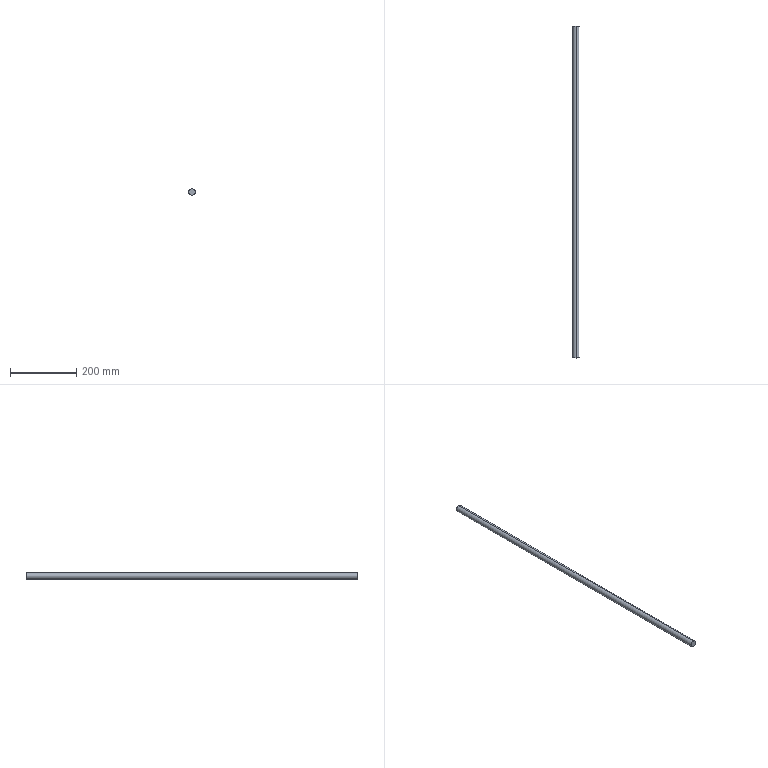Part | SolidWorks | features Extrusion 1 | 1 solid | 4 faces | box 20 x 1000 x 20 mm | volume 314159 mm3 | cylinder 2 | plane 2 | commonest cylinder face diameters 20 x2
STEP:
#1=CARTESIAN_POINT('',(0.,1000.,10.));
#2=VERTEX_POINT('',#1);
#3=CARTESIAN_POINT('',(0.,1000.,-10.));
#4=VERTEX_POINT('',#3);
#5=CARTESIAN_POINT('',(0.,1000.,0.));
#6=DIRECTION('',(0.,1.,0.));
#7=DIRECTION('',(0.,0.,1.));
#8=AXIS2_PLACEMENT_3D('',#5,#6,#7);
#9=CIRCLE('',#8,10.);
#10=EDGE_CURVE('',#2,#4,#9,.T.);
#11=ORIENTED_EDGE('',*,*,#10,.F.);
#12=CARTESIAN_POINT('',(0.,0.,10.));
#13=VERTEX_POINT('',#12);
#14=CARTESIAN_POINT('',(0.,1000.,10.));
#15=DIRECTION('',(0.,-1.,0.));
#16=VECTOR('',#15,1000.);
#17=LINE('',#14,#16);
#18=EDGE_CURVE('',#2,#13,#17,.T.);
#19=ORIENTED_EDGE('',*,*,#18,.T.);
#20=CARTESIAN_POINT('',(0.,0.,-10.));
#21=VERTEX_POINT('',#20);
#22=CARTESIAN_POINT('',(0.,0.,0.));
#23=DIRECTION('',(0.,1.,0.));
#24=DIRECTION('',(0.,0.,1.));
#25=AXIS2_PLACEMENT_3D('',#22,#23,#24);
#26=CIRCLE('',#25,10.);
#27=EDGE_CURVE('',#13,#21,#26,.T.);
#28=ORIENTED_EDGE('',*,*,#27,.T.);
#29=CARTESIAN_POINT('',(0.,1000.,-10.));
#30=DIRECTION('',(0.,-1.,0.));
#31=VECTOR('',#30,1000.);
#32=LINE('',#29,#31);
#33=EDGE_CURVE('',#4,#21,#32,.T.);
#34=ORIENTED_EDGE('',*,*,#33,.F.);
#35=EDGE_LOOP('',(#11,#19,#28,#34));
#36=FACE_OUTER_BOUND('',#35,.T.);
#37=CARTESIAN_POINT('',(0.,1000.,0.));
#38=DIRECTION('',(0.,-1.,0.));
#39=DIRECTION('',(0.,0.,-1.));
#40=AXIS2_PLACEMENT_3D('',#37,#38,#39);
#41=CYLINDRICAL_SURFACE('',#40,10.);
#42=ADVANCED_FACE('',(#36),#41,.T.);
#43=ORIENTED_EDGE('',*,*,#18,.F.);
#44=CARTESIAN_POINT('',(0.,1000.,0.));
#45=DIRECTION('',(0.,1.,0.));
#46=DIRECTION('',(0.,0.,1.));
#47=AXIS2_PLACEMENT_3D('',#44,#45,#46);
#48=CIRCLE('',#47,10.);
#49=EDGE_CURVE('',#4,#2,#48,.T.);
#50=ORIENTED_EDGE('',*,*,#49,.F.);
#51=ORIENTED_EDGE('',*,*,#33,.T.);
#52=CARTESIAN_POINT('',(0.,0.,0.));
#53=DIRECTION('',(0.,1.,0.));
#54=DIRECTION('',(0.,0.,1.));
#55=AXIS2_PLACEMENT_3D('',#52,#53,#54);
#56=CIRCLE('',#55,10.);
#57=EDGE_CURVE('',#21,#13,#56,.T.);
#58=ORIENTED_EDGE('',*,*,#57,.T.);
#59=EDGE_LOOP('',(#43,#50,#51,#58));
#60=FACE_OUTER_BOUND('',#59,.T.);
#61=CARTESIAN_POINT('',(0.,1000.,0.));
#62=DIRECTION('',(0.,-1.,0.));
#63=DIRECTION('',(0.,0.,-1.));
#64=AXIS2_PLACEMENT_3D('',#61,#62,#63);
#65=CYLINDRICAL_SURFACE('',#64,10.);
#66=ADVANCED_FACE('',(#60),#65,.T.);
#67=ORIENTED_EDGE('',*,*,#49,.T.);
#68=ORIENTED_EDGE('',*,*,#10,.T.);
#69=EDGE_LOOP('',(#67,#68));
#70=FACE_OUTER_BOUND('',#69,.T.);
#71=CARTESIAN_POINT('',(0.,1000.,0.));
#72=DIRECTION('',(0.,1.,0.));
#73=DIRECTION('',(0.,0.,1.));
#74=AXIS2_PLACEMENT_3D('',#71,#72,#73);
#75=PLANE('',#74);
#76=ADVANCED_FACE('',(#70),#75,.T.);
#77=ORIENTED_EDGE('',*,*,#57,.F.);
#78=ORIENTED_EDGE('',*,*,#27,.F.);
#79=EDGE_LOOP('',(#77,#78));
#80=FACE_OUTER_BOUND('',#79,.T.);
#81=CARTESIAN_POINT('',(0.,0.,0.));
#82=DIRECTION('',(0.,1.,0.));
#83=DIRECTION('',(0.,0.,1.));
#84=AXIS2_PLACEMENT_3D('',#81,#82,#83);
#85=PLANE('',#84);
#86=ADVANCED_FACE('',(#80),#85,.F.);
#87=CLOSED_SHELL('',(#42,#66,#76,#86));
#88=MANIFOLD_SOLID_BREP('',#87);
#89=CARTESIAN_POINT('',(0.,0.,0.));
#90=DIRECTION('',(0.,0.,1.));
#91=DIRECTION('',(1.,0.,0.));
#92=AXIS2_PLACEMENT_3D('',#89,#90,#91);
#93=(LENGTH_UNIT()NAMED_UNIT(*)SI_UNIT(.MILLI.,.METRE.));
#94=UNCERTAINTY_MEASURE_WITH_UNIT(LENGTH_MEASURE(0.00001),#93,'','');
#95=(NAMED_UNIT(*)PLANE_ANGLE_UNIT()SI_UNIT($,.RADIAN.));
#96=(NAMED_UNIT(*)SI_UNIT($,.STERADIAN.)SOLID_ANGLE_UNIT());
#97=(GEOMETRIC_REPRESENTATION_CONTEXT(3)GLOBAL_UNCERTAINTY_ASSIGNED_CONTEXT((#94))GLOBAL_UNIT_ASSIGNED_CONTEXT((#93,#95,#96))REPRESENTATION_CONTEXT('',''));
#98=ADVANCED_BREP_SHAPE_REPRESENTATION('',(#88,#92),#97);